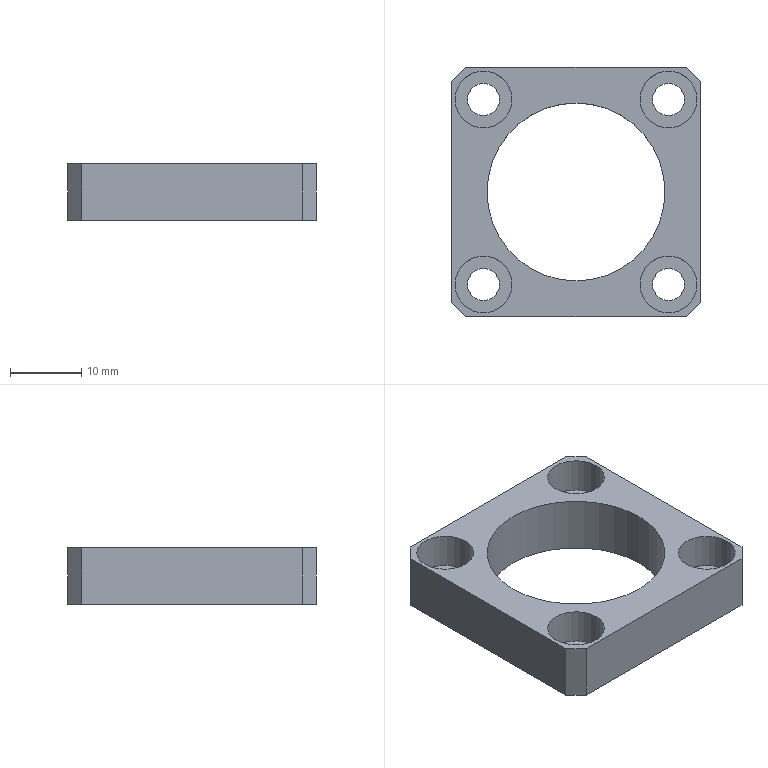Part | NX | 1 solid | 23 faces | box 35 x 35 x 8 mm | volume 4613 mm3 | plane 14 | cylinder 9 | commonest cylinder face diameters 4.5 x4 8 x4 25 x1
STEP:
#1=CARTESIAN_POINT('',(-10.75,13.,0.));
#2=VERTEX_POINT('',#1);
#3=CARTESIAN_POINT('',(-13.,13.,0.));
#4=DIRECTION('',(0.,0.,-1.));
#5=DIRECTION('',(1.,0.,0.));
#6=AXIS2_PLACEMENT_3D('',#3,#4,#5);
#7=CIRCLE('',#6,2.25);
#8=EDGE_CURVE('',#2,#2,#7,.T.);
#9=ORIENTED_EDGE('',*,*,#8,.T.);
#10=EDGE_LOOP('',(#9));
#11=FACE_BOUND('',#10,.T.);
#12=CARTESIAN_POINT('',(-10.75,13.,3.));
#13=VERTEX_POINT('',#12);
#14=CARTESIAN_POINT('',(-13.,13.,3.));
#15=DIRECTION('',(0.,0.,-1.));
#16=DIRECTION('',(1.,0.,0.));
#17=AXIS2_PLACEMENT_3D('',#14,#15,#16);
#18=CIRCLE('',#17,2.25);
#19=EDGE_CURVE('',#13,#13,#18,.T.);
#20=ORIENTED_EDGE('',*,*,#19,.F.);
#21=EDGE_LOOP('',(#20));
#22=FACE_BOUND('',#21,.T.);
#23=CARTESIAN_POINT('',(-13.,13.,8.));
#24=DIRECTION('',(0.,0.,-1.));
#25=DIRECTION('',(1.,0.,0.));
#26=AXIS2_PLACEMENT_3D('',#23,#24,#25);
#27=CYLINDRICAL_SURFACE('',#26,2.25);
#28=ADVANCED_FACE('',(#11,#22),#27,.F.);
#29=CARTESIAN_POINT('',(-15.25,-13.,0.));
#30=VERTEX_POINT('',#29);
#31=CARTESIAN_POINT('',(-13.,-13.,0.));
#32=DIRECTION('',(0.,0.,1.));
#33=DIRECTION('',(-1.,0.,0.));
#34=AXIS2_PLACEMENT_3D('',#31,#32,#33);
#35=CIRCLE('',#34,2.25);
#36=EDGE_CURVE('',#30,#30,#35,.T.);
#37=ORIENTED_EDGE('',*,*,#36,.F.);
#38=EDGE_LOOP('',(#37));
#39=FACE_BOUND('',#38,.T.);
#40=CARTESIAN_POINT('',(-10.75,-13.,3.));
#41=VERTEX_POINT('',#40);
#42=CARTESIAN_POINT('',(-13.,-13.,3.));
#43=DIRECTION('',(0.,0.,1.));
#44=DIRECTION('',(1.,0.,0.));
#45=AXIS2_PLACEMENT_3D('',#42,#43,#44);
#46=CIRCLE('',#45,2.25);
#47=EDGE_CURVE('',#41,#41,#46,.T.);
#48=ORIENTED_EDGE('',*,*,#47,.T.);
#49=EDGE_LOOP('',(#48));
#50=FACE_BOUND('',#49,.T.);
#51=CARTESIAN_POINT('',(-13.,-13.,8.));
#52=DIRECTION('',(0.,0.,-1.));
#53=DIRECTION('',(1.,0.,0.));
#54=AXIS2_PLACEMENT_3D('',#51,#52,#53);
#55=CYLINDRICAL_SURFACE('',#54,2.25);
#56=ADVANCED_FACE('',(#39,#50),#55,.F.);
#57=CARTESIAN_POINT('',(15.25,13.,0.));
#58=VERTEX_POINT('',#57);
#59=CARTESIAN_POINT('',(13.,13.,0.));
#60=DIRECTION('',(0.,0.,1.));
#61=DIRECTION('',(1.,0.,0.));
#62=AXIS2_PLACEMENT_3D('',#59,#60,#61);
#63=CIRCLE('',#62,2.25);
#64=EDGE_CURVE('',#58,#58,#63,.T.);
#65=ORIENTED_EDGE('',*,*,#64,.F.);
#66=EDGE_LOOP('',(#65));
#67=FACE_BOUND('',#66,.T.);
#68=CARTESIAN_POINT('',(15.25,13.,3.));
#69=VERTEX_POINT('',#68);
#70=CARTESIAN_POINT('',(13.,13.,3.));
#71=DIRECTION('',(0.,0.,1.));
#72=DIRECTION('',(1.,0.,0.));
#73=AXIS2_PLACEMENT_3D('',#70,#71,#72);
#74=CIRCLE('',#73,2.25);
#75=EDGE_CURVE('',#69,#69,#74,.T.);
#76=ORIENTED_EDGE('',*,*,#75,.T.);
#77=EDGE_LOOP('',(#76));
#78=FACE_BOUND('',#77,.T.);
#79=CARTESIAN_POINT('',(13.,13.,8.));
#80=DIRECTION('',(0.,0.,-1.));
#81=DIRECTION('',(1.,0.,0.));
#82=AXIS2_PLACEMENT_3D('',#79,#80,#81);
#83=CYLINDRICAL_SURFACE('',#82,2.25);
#84=ADVANCED_FACE('',(#67,#78),#83,.F.);
#85=CARTESIAN_POINT('',(10.75,-13.,0.));
#86=VERTEX_POINT('',#85);
#87=CARTESIAN_POINT('',(13.,-13.,0.));
#88=DIRECTION('',(0.,0.,-1.));
#89=DIRECTION('',(-1.,0.,0.));
#90=AXIS2_PLACEMENT_3D('',#87,#88,#89);
#91=CIRCLE('',#90,2.25);
#92=EDGE_CURVE('',#86,#86,#91,.T.);
#93=ORIENTED_EDGE('',*,*,#92,.T.);
#94=EDGE_LOOP('',(#93));
#95=FACE_BOUND('',#94,.T.);
#96=CARTESIAN_POINT('',(15.25,-13.,3.));
#97=VERTEX_POINT('',#96);
#98=CARTESIAN_POINT('',(13.,-13.,3.));
#99=DIRECTION('',(0.,0.,-1.));
#100=DIRECTION('',(1.,0.,0.));
#101=AXIS2_PLACEMENT_3D('',#98,#99,#100);
#102=CIRCLE('',#101,2.25);
#103=EDGE_CURVE('',#97,#97,#102,.T.);
#104=ORIENTED_EDGE('',*,*,#103,.F.);
#105=EDGE_LOOP('',(#104));
#106=FACE_BOUND('',#105,.T.);
#107=CARTESIAN_POINT('',(13.,-13.,8.));
#108=DIRECTION('',(0.,0.,-1.));
#109=DIRECTION('',(1.,0.,0.));
#110=AXIS2_PLACEMENT_3D('',#107,#108,#109);
#111=CYLINDRICAL_SURFACE('',#110,2.25);
#112=ADVANCED_FACE('',(#95,#106),#111,.F.);
#113=CARTESIAN_POINT('',(-17.5,-15.5,0.));
#114=VERTEX_POINT('',#113);
#115=CARTESIAN_POINT('',(-17.5,15.5,0.));
#116=VERTEX_POINT('',#115);
#117=CARTESIAN_POINT('',(-17.5,-15.5,0.));
#118=DIRECTION('',(0.,1.,0.));
#119=VECTOR('',#118,1.);
#120=LINE('',#117,#119);
#121=EDGE_CURVE('',#114,#116,#120,.T.);
#122=ORIENTED_EDGE('',*,*,#121,.F.);
#123=CARTESIAN_POINT('',(-17.5,-15.5,8.));
#124=VERTEX_POINT('',#123);
#125=CARTESIAN_POINT('',(-17.5,-15.5,8.));
#126=DIRECTION('',(0.,0.,-1.));
#127=VECTOR('',#126,1.);
#128=LINE('',#125,#127);
#129=EDGE_CURVE('',#124,#114,#128,.T.);
#130=ORIENTED_EDGE('',*,*,#129,.F.);
#131=CARTESIAN_POINT('',(-17.5,15.5,8.));
#132=VERTEX_POINT('',#131);
#133=CARTESIAN_POINT('',(-17.5,-15.5,8.));
#134=DIRECTION('',(0.,1.,0.));
#135=VECTOR('',#134,1.);
#136=LINE('',#133,#135);
#137=EDGE_CURVE('',#124,#132,#136,.T.);
#138=ORIENTED_EDGE('',*,*,#137,.T.);
#139=CARTESIAN_POINT('',(-17.5,15.5,8.));
#140=DIRECTION('',(0.,0.,-1.));
#141=VECTOR('',#140,1.);
#142=LINE('',#139,#141);
#143=EDGE_CURVE('',#132,#116,#142,.T.);
#144=ORIENTED_EDGE('',*,*,#143,.T.);
#145=EDGE_LOOP('',(#122,#130,#138,#144));
#146=FACE_OUTER_BOUND('',#145,.T.);
#147=CARTESIAN_POINT('',(-17.5,-15.5,8.));
#148=DIRECTION('',(-1.,0.,0.));
#149=DIRECTION('',(0.,0.,-1.));
#150=AXIS2_PLACEMENT_3D('',#147,#148,#149);
#151=PLANE('',#150);
#152=ADVANCED_FACE('',(#146),#151,.T.);
#153=CARTESIAN_POINT('',(-15.5,17.5,0.));
#154=VERTEX_POINT('',#153);
#155=CARTESIAN_POINT('',(-17.5,15.5,0.));
#156=DIRECTION('',(0.7071,0.7071,0.));
#157=VECTOR('',#156,1.);
#158=LINE('',#155,#157);
#159=EDGE_CURVE('',#116,#154,#158,.T.);
#160=ORIENTED_EDGE('',*,*,#159,.F.);
#161=ORIENTED_EDGE('',*,*,#143,.F.);
#162=CARTESIAN_POINT('',(-15.5,17.5,8.));
#163=VERTEX_POINT('',#162);
#164=CARTESIAN_POINT('',(-17.5,15.5,8.));
#165=DIRECTION('',(0.7071,0.7071,0.));
#166=VECTOR('',#165,1.);
#167=LINE('',#164,#166);
#168=EDGE_CURVE('',#132,#163,#167,.T.);
#169=ORIENTED_EDGE('',*,*,#168,.T.);
#170=CARTESIAN_POINT('',(-15.5,17.5,8.));
#171=DIRECTION('',(0.,0.,-1.));
#172=VECTOR('',#171,1.);
#173=LINE('',#170,#172);
#174=EDGE_CURVE('',#163,#154,#173,.T.);
#175=ORIENTED_EDGE('',*,*,#174,.T.);
#176=EDGE_LOOP('',(#160,#161,#169,#175));
#177=FACE_OUTER_BOUND('',#176,.T.);
#178=CARTESIAN_POINT('',(-17.5,15.5,8.));
#179=DIRECTION('',(-0.7071,0.7071,0.));
#180=DIRECTION('',(0.7071,0.7071,0.));
#181=AXIS2_PLACEMENT_3D('',#178,#179,#180);
#182=PLANE('',#181);
#183=ADVANCED_FACE('',(#177),#182,.T.);
#184=CARTESIAN_POINT('',(15.5,17.5,0.));
#185=VERTEX_POINT('',#184);
#186=CARTESIAN_POINT('',(-15.5,17.5,0.));
#187=DIRECTION('',(1.,0.,0.));
#188=VECTOR('',#187,1.);
#189=LINE('',#186,#188);
#190=EDGE_CURVE('',#154,#185,#189,.T.);
#191=ORIENTED_EDGE('',*,*,#190,.F.);
#192=ORIENTED_EDGE('',*,*,#174,.F.);
#193=CARTESIAN_POINT('',(15.5,17.5,8.));
#194=VERTEX_POINT('',#193);
#195=CARTESIAN_POINT('',(-15.5,17.5,8.));
#196=DIRECTION('',(1.,0.,0.));
#197=VECTOR('',#196,1.);
#198=LINE('',#195,#197);
#199=EDGE_CURVE('',#163,#194,#198,.T.);
#200=ORIENTED_EDGE('',*,*,#199,.T.);
#201=CARTESIAN_POINT('',(15.5,17.5,8.));
#202=DIRECTION('',(0.,0.,-1.));
#203=VECTOR('',#202,1.);
#204=LINE('',#201,#203);
#205=EDGE_CURVE('',#194,#185,#204,.T.);
#206=ORIENTED_EDGE('',*,*,#205,.T.);
#207=EDGE_LOOP('',(#191,#192,#200,#206));
#208=FACE_OUTER_BOUND('',#207,.T.);
#209=CARTESIAN_POINT('',(-15.5,17.5,8.));
#210=DIRECTION('',(0.,1.,0.));
#211=DIRECTION('',(0.,0.,-1.));
#212=AXIS2_PLACEMENT_3D('',#209,#210,#211);
#213=PLANE('',#212);
#214=ADVANCED_FACE('',(#208),#213,.T.);
#215=CARTESIAN_POINT('',(17.5,15.5,0.));
#216=VERTEX_POINT('',#215);
#217=CARTESIAN_POINT('',(15.5,17.5,0.));
#218=DIRECTION('',(0.7071,-0.7071,0.));
#219=VECTOR('',#218,1.);
#220=LINE('',#217,#219);
#221=EDGE_CURVE('',#185,#216,#220,.T.);
#222=ORIENTED_EDGE('',*,*,#221,.F.);
#223=ORIENTED_EDGE('',*,*,#205,.F.);
#224=CARTESIAN_POINT('',(17.5,15.5,8.));
#225=VERTEX_POINT('',#224);
#226=CARTESIAN_POINT('',(15.5,17.5,8.));
#227=DIRECTION('',(0.7071,-0.7071,0.));
#228=VECTOR('',#227,1.);
#229=LINE('',#226,#228);
#230=EDGE_CURVE('',#194,#225,#229,.T.);
#231=ORIENTED_EDGE('',*,*,#230,.T.);
#232=CARTESIAN_POINT('',(17.5,15.5,8.));
#233=DIRECTION('',(0.,0.,-1.));
#234=VECTOR('',#233,1.);
#235=LINE('',#232,#234);
#236=EDGE_CURVE('',#225,#216,#235,.T.);
#237=ORIENTED_EDGE('',*,*,#236,.T.);
#238=EDGE_LOOP('',(#222,#223,#231,#237));
#239=FACE_OUTER_BOUND('',#238,.T.);
#240=CARTESIAN_POINT('',(15.5,17.5,8.));
#241=DIRECTION('',(0.7071,0.7071,0.));
#242=DIRECTION('',(0.7071,-0.7071,0.));
#243=AXIS2_PLACEMENT_3D('',#240,#241,#242);
#244=PLANE('',#243);
#245=ADVANCED_FACE('',(#239),#244,.T.);
#246=CARTESIAN_POINT('',(17.5,-15.5,0.));
#247=VERTEX_POINT('',#246);
#248=CARTESIAN_POINT('',(17.5,15.5,0.));
#249=DIRECTION('',(0.,-1.,0.));
#250=VECTOR('',#249,1.);
#251=LINE('',#248,#250);
#252=EDGE_CURVE('',#216,#247,#251,.T.);
#253=ORIENTED_EDGE('',*,*,#252,.F.);
#254=ORIENTED_EDGE('',*,*,#236,.F.);
#255=CARTESIAN_POINT('',(17.5,-15.5,8.));
#256=VERTEX_POINT('',#255);
#257=CARTESIAN_POINT('',(17.5,15.5,8.));
#258=DIRECTION('',(0.,-1.,0.));
#259=VECTOR('',#258,1.);
#260=LINE('',#257,#259);
#261=EDGE_CURVE('',#225,#256,#260,.T.);
#262=ORIENTED_EDGE('',*,*,#261,.T.);
#263=CARTESIAN_POINT('',(17.5,-15.5,8.));
#264=DIRECTION('',(0.,0.,-1.));
#265=VECTOR('',#264,1.);
#266=LINE('',#263,#265);
#267=EDGE_CURVE('',#256,#247,#266,.T.);
#268=ORIENTED_EDGE('',*,*,#267,.T.);
#269=EDGE_LOOP('',(#253,#254,#262,#268));
#270=FACE_OUTER_BOUND('',#269,.T.);
#271=CARTESIAN_POINT('',(17.5,15.5,8.));
#272=DIRECTION('',(1.,0.,0.));
#273=DIRECTION('',(0.,0.,1.));
#274=AXIS2_PLACEMENT_3D('',#271,#272,#273);
#275=PLANE('',#274);
#276=ADVANCED_FACE('',(#270),#275,.T.);
#277=CARTESIAN_POINT('',(15.5,-17.5,0.));
#278=VERTEX_POINT('',#277);
#279=CARTESIAN_POINT('',(17.5,-15.5,0.));
#280=DIRECTION('',(-0.7071,-0.7071,0.));
#281=VECTOR('',#280,1.);
#282=LINE('',#279,#281);
#283=EDGE_CURVE('',#247,#278,#282,.T.);
#284=ORIENTED_EDGE('',*,*,#283,.F.);
#285=ORIENTED_EDGE('',*,*,#267,.F.);
#286=CARTESIAN_POINT('',(15.5,-17.5,8.));
#287=VERTEX_POINT('',#286);
#288=CARTESIAN_POINT('',(17.5,-15.5,8.));
#289=DIRECTION('',(-0.7071,-0.7071,0.));
#290=VECTOR('',#289,1.);
#291=LINE('',#288,#290);
#292=EDGE_CURVE('',#256,#287,#291,.T.);
#293=ORIENTED_EDGE('',*,*,#292,.T.);
#294=CARTESIAN_POINT('',(15.5,-17.5,8.));
#295=DIRECTION('',(0.,0.,-1.));
#296=VECTOR('',#295,1.);
#297=LINE('',#294,#296);
#298=EDGE_CURVE('',#287,#278,#297,.T.);
#299=ORIENTED_EDGE('',*,*,#298,.T.);
#300=EDGE_LOOP('',(#284,#285,#293,#299));
#301=FACE_OUTER_BOUND('',#300,.T.);
#302=CARTESIAN_POINT('',(17.5,-15.5,8.));
#303=DIRECTION('',(0.7071,-0.7071,0.));
#304=DIRECTION('',(-0.7071,-0.7071,0.));
#305=AXIS2_PLACEMENT_3D('',#302,#303,#304);
#306=PLANE('',#305);
#307=ADVANCED_FACE('',(#301),#306,.T.);
#308=CARTESIAN_POINT('',(-15.5,-17.5,0.));
#309=VERTEX_POINT('',#308);
#310=CARTESIAN_POINT('',(15.5,-17.5,0.));
#311=DIRECTION('',(-1.,0.,0.));
#312=VECTOR('',#311,1.);
#313=LINE('',#310,#312);
#314=EDGE_CURVE('',#278,#309,#313,.T.);
#315=ORIENTED_EDGE('',*,*,#314,.F.);
#316=ORIENTED_EDGE('',*,*,#298,.F.);
#317=CARTESIAN_POINT('',(-15.5,-17.5,8.));
#318=VERTEX_POINT('',#317);
#319=CARTESIAN_POINT('',(15.5,-17.5,8.));
#320=DIRECTION('',(-1.,0.,0.));
#321=VECTOR('',#320,1.);
#322=LINE('',#319,#321);
#323=EDGE_CURVE('',#287,#318,#322,.T.);
#324=ORIENTED_EDGE('',*,*,#323,.T.);
#325=CARTESIAN_POINT('',(-15.5,-17.5,8.));
#326=DIRECTION('',(0.,0.,-1.));
#327=VECTOR('',#326,1.);
#328=LINE('',#325,#327);
#329=EDGE_CURVE('',#318,#309,#328,.T.);
#330=ORIENTED_EDGE('',*,*,#329,.T.);
#331=EDGE_LOOP('',(#315,#316,#324,#330));
#332=FACE_OUTER_BOUND('',#331,.T.);
#333=CARTESIAN_POINT('',(15.5,-17.5,8.));
#334=DIRECTION('',(0.,-1.,0.));
#335=DIRECTION('',(0.,0.,1.));
#336=AXIS2_PLACEMENT_3D('',#333,#334,#335);
#337=PLANE('',#336);
#338=ADVANCED_FACE('',(#332),#337,.T.);
#339=CARTESIAN_POINT('',(12.5,0.,0.));
#340=VERTEX_POINT('',#339);
#341=CARTESIAN_POINT('',(0.,0.,0.));
#342=DIRECTION('',(0.,0.,1.));
#343=DIRECTION('',(1.,0.,0.));
#344=AXIS2_PLACEMENT_3D('',#341,#342,#343);
#345=CIRCLE('',#344,12.5);
#346=EDGE_CURVE('',#340,#340,#345,.T.);
#347=ORIENTED_EDGE('',*,*,#346,.F.);
#348=EDGE_LOOP('',(#347));
#349=FACE_BOUND('',#348,.T.);
#350=CARTESIAN_POINT('',(12.5,0.,8.));
#351=VERTEX_POINT('',#350);
#352=CARTESIAN_POINT('',(0.,0.,8.));
#353=DIRECTION('',(0.,0.,1.));
#354=DIRECTION('',(1.,0.,0.));
#355=AXIS2_PLACEMENT_3D('',#352,#353,#354);
#356=CIRCLE('',#355,12.5);
#357=EDGE_CURVE('',#351,#351,#356,.T.);
#358=ORIENTED_EDGE('',*,*,#357,.T.);
#359=EDGE_LOOP('',(#358));
#360=FACE_BOUND('',#359,.T.);
#361=CARTESIAN_POINT('',(0.,0.,8.));
#362=DIRECTION('',(0.,0.,-1.));
#363=DIRECTION('',(1.,0.,0.));
#364=AXIS2_PLACEMENT_3D('',#361,#362,#363);
#365=CYLINDRICAL_SURFACE('',#364,12.5);
#366=ADVANCED_FACE('',(#349,#360),#365,.F.);
#367=CARTESIAN_POINT('',(-15.5,-17.5,0.));
#368=DIRECTION('',(-0.7071,0.7071,0.));
#369=VECTOR('',#368,1.);
#370=LINE('',#367,#369);
#371=EDGE_CURVE('',#309,#114,#370,.T.);
#372=ORIENTED_EDGE('',*,*,#371,.F.);
#373=ORIENTED_EDGE('',*,*,#329,.F.);
#374=CARTESIAN_POINT('',(-15.5,-17.5,8.));
#375=DIRECTION('',(-0.7071,0.7071,0.));
#376=VECTOR('',#375,1.);
#377=LINE('',#374,#376);
#378=EDGE_CURVE('',#318,#124,#377,.T.);
#379=ORIENTED_EDGE('',*,*,#378,.T.);
#380=ORIENTED_EDGE('',*,*,#129,.T.);
#381=EDGE_LOOP('',(#372,#373,#379,#380));
#382=FACE_OUTER_BOUND('',#381,.T.);
#383=CARTESIAN_POINT('',(-15.5,-17.5,8.));
#384=DIRECTION('',(-0.7071,-0.7071,0.));
#385=DIRECTION('',(-0.7071,0.7071,0.));
#386=AXIS2_PLACEMENT_3D('',#383,#384,#385);
#387=PLANE('',#386);
#388=ADVANCED_FACE('',(#382),#387,.T.);
#389=CARTESIAN_POINT('',(17.,-13.,8.));
#390=VERTEX_POINT('',#389);
#391=CARTESIAN_POINT('',(13.,-13.,8.));
#392=DIRECTION('',(0.,0.,1.));
#393=DIRECTION('',(1.,0.,0.));
#394=AXIS2_PLACEMENT_3D('',#391,#392,#393);
#395=CIRCLE('',#394,4.);
#396=EDGE_CURVE('',#390,#390,#395,.T.);
#397=ORIENTED_EDGE('',*,*,#396,.F.);
#398=EDGE_LOOP('',(#397));
#399=FACE_BOUND('',#398,.T.);
#400=CARTESIAN_POINT('',(-9.,13.,8.));
#401=VERTEX_POINT('',#400);
#402=CARTESIAN_POINT('',(-13.,13.,8.));
#403=DIRECTION('',(0.,0.,1.));
#404=DIRECTION('',(1.,0.,0.));
#405=AXIS2_PLACEMENT_3D('',#402,#403,#404);
#406=CIRCLE('',#405,4.);
#407=EDGE_CURVE('',#401,#401,#406,.T.);
#408=ORIENTED_EDGE('',*,*,#407,.F.);
#409=EDGE_LOOP('',(#408));
#410=FACE_BOUND('',#409,.T.);
#411=CARTESIAN_POINT('',(-9.,-13.,8.));
#412=VERTEX_POINT('',#411);
#413=CARTESIAN_POINT('',(-13.,-13.,8.));
#414=DIRECTION('',(0.,0.,1.));
#415=DIRECTION('',(1.,0.,0.));
#416=AXIS2_PLACEMENT_3D('',#413,#414,#415);
#417=CIRCLE('',#416,4.);
#418=EDGE_CURVE('',#412,#412,#417,.T.);
#419=ORIENTED_EDGE('',*,*,#418,.F.);
#420=EDGE_LOOP('',(#419));
#421=FACE_BOUND('',#420,.T.);
#422=CARTESIAN_POINT('',(17.,13.,8.));
#423=VERTEX_POINT('',#422);
#424=CARTESIAN_POINT('',(13.,13.,8.));
#425=DIRECTION('',(0.,0.,1.));
#426=DIRECTION('',(1.,0.,0.));
#427=AXIS2_PLACEMENT_3D('',#424,#425,#426);
#428=CIRCLE('',#427,4.);
#429=EDGE_CURVE('',#423,#423,#428,.T.);
#430=ORIENTED_EDGE('',*,*,#429,.F.);
#431=EDGE_LOOP('',(#430));
#432=FACE_BOUND('',#431,.T.);
#433=ORIENTED_EDGE('',*,*,#137,.F.);
#434=ORIENTED_EDGE('',*,*,#378,.F.);
#435=ORIENTED_EDGE('',*,*,#323,.F.);
#436=ORIENTED_EDGE('',*,*,#292,.F.);
#437=ORIENTED_EDGE('',*,*,#261,.F.);
#438=ORIENTED_EDGE('',*,*,#230,.F.);
#439=ORIENTED_EDGE('',*,*,#199,.F.);
#440=ORIENTED_EDGE('',*,*,#168,.F.);
#441=EDGE_LOOP('',(#433,#434,#435,#436,#437,#438,#439,#440));
#442=FACE_BOUND('',#441,.T.);
#443=ORIENTED_EDGE('',*,*,#357,.F.);
#444=EDGE_LOOP('',(#443));
#445=FACE_BOUND('',#444,.T.);
#446=CARTESIAN_POINT('',(13.,13.,8.));
#447=DIRECTION('',(0.,0.,1.));
#448=DIRECTION('',(-1.,0.,0.));
#449=AXIS2_PLACEMENT_3D('',#446,#447,#448);
#450=PLANE('',#449);
#451=ADVANCED_FACE('',(#399,#410,#421,#432,#442,#445),#450,.T.);
#452=ORIENTED_EDGE('',*,*,#121,.T.);
#453=ORIENTED_EDGE('',*,*,#159,.T.);
#454=ORIENTED_EDGE('',*,*,#190,.T.);
#455=ORIENTED_EDGE('',*,*,#221,.T.);
#456=ORIENTED_EDGE('',*,*,#252,.T.);
#457=ORIENTED_EDGE('',*,*,#283,.T.);
#458=ORIENTED_EDGE('',*,*,#314,.T.);
#459=ORIENTED_EDGE('',*,*,#371,.T.);
#460=EDGE_LOOP('',(#452,#453,#454,#455,#456,#457,#458,#459));
#461=FACE_BOUND('',#460,.T.);
#462=ORIENTED_EDGE('',*,*,#64,.T.);
#463=EDGE_LOOP('',(#462));
#464=FACE_BOUND('',#463,.T.);
#465=ORIENTED_EDGE('',*,*,#346,.T.);
#466=EDGE_LOOP('',(#465));
#467=FACE_BOUND('',#466,.T.);
#468=ORIENTED_EDGE('',*,*,#36,.T.);
#469=EDGE_LOOP('',(#468));
#470=FACE_BOUND('',#469,.T.);
#471=ORIENTED_EDGE('',*,*,#8,.F.);
#472=EDGE_LOOP('',(#471));
#473=FACE_BOUND('',#472,.T.);
#474=ORIENTED_EDGE('',*,*,#92,.F.);
#475=EDGE_LOOP('',(#474));
#476=FACE_BOUND('',#475,.T.);
#477=CARTESIAN_POINT('',(13.,13.,0.));
#478=DIRECTION('',(0.,0.,1.));
#479=DIRECTION('',(-1.,0.,0.));
#480=AXIS2_PLACEMENT_3D('',#477,#478,#479);
#481=PLANE('',#480);
#482=ADVANCED_FACE('',(#461,#464,#467,#470,#473,#476),#481,.F.);
#483=CARTESIAN_POINT('',(17.,13.,3.));
#484=VERTEX_POINT('',#483);
#485=CARTESIAN_POINT('',(13.,13.,3.));
#486=DIRECTION('',(0.,0.,-1.));
#487=DIRECTION('',(1.,0.,0.));
#488=AXIS2_PLACEMENT_3D('',#485,#486,#487);
#489=CIRCLE('',#488,4.);
#490=EDGE_CURVE('',#484,#484,#489,.T.);
#491=ORIENTED_EDGE('',*,*,#490,.T.);
#492=EDGE_LOOP('',(#491));
#493=FACE_BOUND('',#492,.T.);
#494=ORIENTED_EDGE('',*,*,#429,.T.);
#495=EDGE_LOOP('',(#494));
#496=FACE_BOUND('',#495,.T.);
#497=CARTESIAN_POINT('',(13.,13.,8.));
#498=DIRECTION('',(0.,0.,-1.));
#499=DIRECTION('',(1.,0.,0.));
#500=AXIS2_PLACEMENT_3D('',#497,#498,#499);
#501=CYLINDRICAL_SURFACE('',#500,4.);
#502=ADVANCED_FACE('',(#493,#496),#501,.F.);
#503=ORIENTED_EDGE('',*,*,#75,.F.);
#504=EDGE_LOOP('',(#503));
#505=FACE_BOUND('',#504,.T.);
#506=ORIENTED_EDGE('',*,*,#490,.F.);
#507=EDGE_LOOP('',(#506));
#508=FACE_BOUND('',#507,.T.);
#509=CARTESIAN_POINT('',(13.,13.,3.));
#510=DIRECTION('',(0.,0.,1.));
#511=DIRECTION('',(-1.,0.,0.));
#512=AXIS2_PLACEMENT_3D('',#509,#510,#511);
#513=PLANE('',#512);
#514=ADVANCED_FACE('',(#505,#508),#513,.T.);
#515=CARTESIAN_POINT('',(-9.,-13.,3.));
#516=VERTEX_POINT('',#515);
#517=CARTESIAN_POINT('',(-13.,-13.,3.));
#518=DIRECTION('',(0.,0.,-1.));
#519=DIRECTION('',(1.,0.,0.));
#520=AXIS2_PLACEMENT_3D('',#517,#518,#519);
#521=CIRCLE('',#520,4.);
#522=EDGE_CURVE('',#516,#516,#521,.T.);
#523=ORIENTED_EDGE('',*,*,#522,.T.);
#524=EDGE_LOOP('',(#523));
#525=FACE_BOUND('',#524,.T.);
#526=ORIENTED_EDGE('',*,*,#418,.T.);
#527=EDGE_LOOP('',(#526));
#528=FACE_BOUND('',#527,.T.);
#529=CARTESIAN_POINT('',(-13.,-13.,8.));
#530=DIRECTION('',(0.,0.,-1.));
#531=DIRECTION('',(1.,0.,0.));
#532=AXIS2_PLACEMENT_3D('',#529,#530,#531);
#533=CYLINDRICAL_SURFACE('',#532,4.);
#534=ADVANCED_FACE('',(#525,#528),#533,.F.);
#535=ORIENTED_EDGE('',*,*,#47,.F.);
#536=EDGE_LOOP('',(#535));
#537=FACE_BOUND('',#536,.T.);
#538=ORIENTED_EDGE('',*,*,#522,.F.);
#539=EDGE_LOOP('',(#538));
#540=FACE_BOUND('',#539,.T.);
#541=CARTESIAN_POINT('',(-13.,-13.,3.));
#542=DIRECTION('',(0.,0.,1.));
#543=DIRECTION('',(-1.,0.,0.));
#544=AXIS2_PLACEMENT_3D('',#541,#542,#543);
#545=PLANE('',#544);
#546=ADVANCED_FACE('',(#537,#540),#545,.T.);
#547=CARTESIAN_POINT('',(-9.,13.,3.));
#548=VERTEX_POINT('',#547);
#549=CARTESIAN_POINT('',(-13.,13.,3.));
#550=DIRECTION('',(0.,0.,-1.));
#551=DIRECTION('',(1.,0.,0.));
#552=AXIS2_PLACEMENT_3D('',#549,#550,#551);
#553=CIRCLE('',#552,4.);
#554=EDGE_CURVE('',#548,#548,#553,.T.);
#555=ORIENTED_EDGE('',*,*,#554,.F.);
#556=EDGE_LOOP('',(#555));
#557=FACE_BOUND('',#556,.T.);
#558=ORIENTED_EDGE('',*,*,#19,.T.);
#559=EDGE_LOOP('',(#558));
#560=FACE_BOUND('',#559,.T.);
#561=CARTESIAN_POINT('',(-13.,13.,3.));
#562=DIRECTION('',(0.,0.,1.));
#563=DIRECTION('',(-1.,0.,0.));
#564=AXIS2_PLACEMENT_3D('',#561,#562,#563);
#565=PLANE('',#564);
#566=ADVANCED_FACE('',(#557,#560),#565,.T.);
#567=ORIENTED_EDGE('',*,*,#554,.T.);
#568=EDGE_LOOP('',(#567));
#569=FACE_BOUND('',#568,.T.);
#570=ORIENTED_EDGE('',*,*,#407,.T.);
#571=EDGE_LOOP('',(#570));
#572=FACE_BOUND('',#571,.T.);
#573=CARTESIAN_POINT('',(-13.,13.,8.));
#574=DIRECTION('',(0.,0.,-1.));
#575=DIRECTION('',(1.,0.,0.));
#576=AXIS2_PLACEMENT_3D('',#573,#574,#575);
#577=CYLINDRICAL_SURFACE('',#576,4.);
#578=ADVANCED_FACE('',(#569,#572),#577,.F.);
#579=CARTESIAN_POINT('',(17.,-13.,3.));
#580=VERTEX_POINT('',#579);
#581=CARTESIAN_POINT('',(13.,-13.,3.));
#582=DIRECTION('',(0.,0.,-1.));
#583=DIRECTION('',(1.,0.,0.));
#584=AXIS2_PLACEMENT_3D('',#581,#582,#583);
#585=CIRCLE('',#584,4.);
#586=EDGE_CURVE('',#580,#580,#585,.T.);
#587=ORIENTED_EDGE('',*,*,#586,.F.);
#588=EDGE_LOOP('',(#587));
#589=FACE_BOUND('',#588,.T.);
#590=ORIENTED_EDGE('',*,*,#103,.T.);
#591=EDGE_LOOP('',(#590));
#592=FACE_BOUND('',#591,.T.);
#593=CARTESIAN_POINT('',(13.,-13.,3.));
#594=DIRECTION('',(0.,0.,1.));
#595=DIRECTION('',(-1.,0.,0.));
#596=AXIS2_PLACEMENT_3D('',#593,#594,#595);
#597=PLANE('',#596);
#598=ADVANCED_FACE('',(#589,#592),#597,.T.);
#599=ORIENTED_EDGE('',*,*,#586,.T.);
#600=EDGE_LOOP('',(#599));
#601=FACE_BOUND('',#600,.T.);
#602=ORIENTED_EDGE('',*,*,#396,.T.);
#603=EDGE_LOOP('',(#602));
#604=FACE_BOUND('',#603,.T.);
#605=CARTESIAN_POINT('',(13.,-13.,8.));
#606=DIRECTION('',(0.,0.,-1.));
#607=DIRECTION('',(1.,0.,0.));
#608=AXIS2_PLACEMENT_3D('',#605,#606,#607);
#609=CYLINDRICAL_SURFACE('',#608,4.);
#610=ADVANCED_FACE('',(#601,#604),#609,.F.);
#611=CLOSED_SHELL('',(#28,#56,#84,#112,#152,#183,#214,#245,#276,#307,#338,#366,#388,#451,#482,#502,#514,#534,#546,#566,#578,#598,#610));
#612=MANIFOLD_SOLID_BREP('',#611);
#613=(LENGTH_UNIT()NAMED_UNIT(*)SI_UNIT(.MILLI.,.METRE.));
#614=UNCERTAINTY_MEASURE_WITH_UNIT(LENGTH_MEASURE(0.00002),#613,'','');
#615=(NAMED_UNIT(*)PLANE_ANGLE_UNIT()SI_UNIT($,.RADIAN.));
#616=PLANE_ANGLE_MEASURE_WITH_UNIT(PLANE_ANGLE_MEASURE(0.01745),#615);
#617=DIMENSIONAL_EXPONENTS(0.,0.,0.,0.,0.,0.,0.);
#618=(CONVERSION_BASED_UNIT('DEGREE',#616)NAMED_UNIT(#617)PLANE_ANGLE_UNIT());
#619=(NAMED_UNIT(*)SI_UNIT($,.STERADIAN.)SOLID_ANGLE_UNIT());
#620=(GEOMETRIC_REPRESENTATION_CONTEXT(3)GLOBAL_UNCERTAINTY_ASSIGNED_CONTEXT((#614))GLOBAL_UNIT_ASSIGNED_CONTEXT((#613,#618,#619))REPRESENTATION_CONTEXT('',''));
#621=ADVANCED_BREP_SHAPE_REPRESENTATION('',(#612),#620);